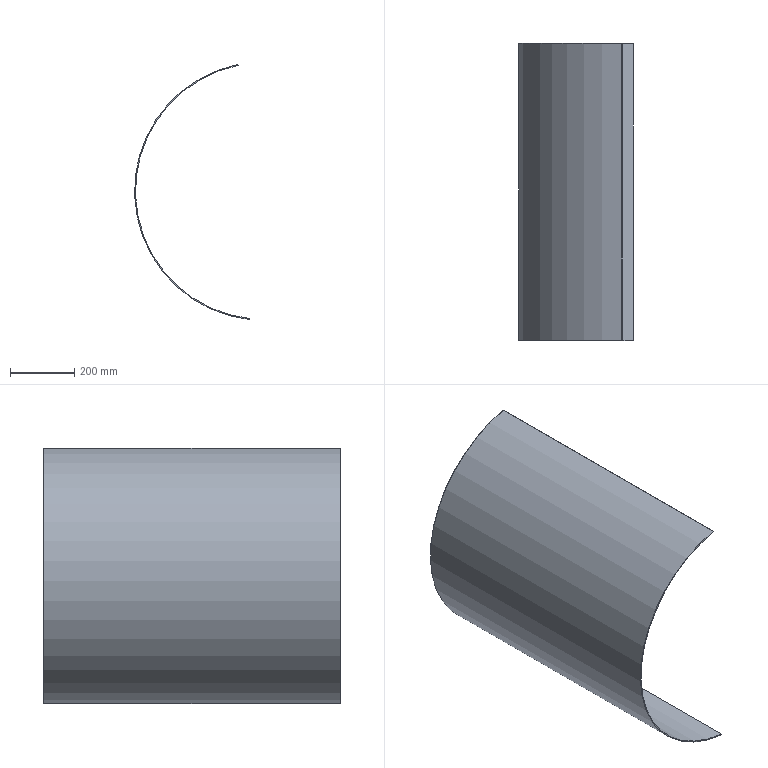Part | NX | features DATUM_CSYS 2, EXTRUDE 1, SKETCH 1 | 1 solid | 6 faces | box 358 x 926 x 795.299 mm | volume 3153696 mm3 | plane 4 | cylinder 2 | commonest cylinder face diameters 800 x1 806 x1
STEP:
#1=CARTESIAN_POINT('',(-80.,463.,391.918));
#2=VERTEX_POINT('',#1);
#3=CARTESIAN_POINT('',(-80.6,463.,394.858));
#4=VERTEX_POINT('',#3);
#5=CARTESIAN_POINT('',(-80.,463.,391.918));
#6=DIRECTION('',(-0.2,0.,0.9798));
#7=VECTOR('',#6,1000.);
#8=LINE('',#5,#7);
#9=EDGE_CURVE('',#2,#4,#8,.T.);
#10=ORIENTED_EDGE('',*,*,#9,.F.);
#11=CARTESIAN_POINT('',(-45.,463.,-397.461));
#12=VERTEX_POINT('',#11);
#13=CARTESIAN_POINT('',(0.,463.,0.));
#14=DIRECTION('',(0.,-1.,0.));
#15=DIRECTION('',(1.,0.,0.));
#16=AXIS2_PLACEMENT_3D('',#13,#14,#15);
#17=CIRCLE('',#16,400.);
#18=EDGE_CURVE('',#2,#12,#17,.T.);
#19=ORIENTED_EDGE('',*,*,#18,.T.);
#20=CARTESIAN_POINT('',(-45.338,463.,-400.442));
#21=VERTEX_POINT('',#20);
#22=CARTESIAN_POINT('',(-45.,463.,-397.461));
#23=DIRECTION('',(-0.1125,0.,-0.9937));
#24=VECTOR('',#23,1000.);
#25=LINE('',#22,#24);
#26=EDGE_CURVE('',#12,#21,#25,.T.);
#27=ORIENTED_EDGE('',*,*,#26,.T.);
#28=CARTESIAN_POINT('',(0.,463.,0.));
#29=DIRECTION('',(0.,-1.,0.));
#30=DIRECTION('',(0.,0.,-1.));
#31=AXIS2_PLACEMENT_3D('',#28,#29,#30);
#32=CIRCLE('',#31,403.);
#33=EDGE_CURVE('',#4,#21,#32,.T.);
#34=ORIENTED_EDGE('',*,*,#33,.F.);
#35=EDGE_LOOP('',(#10,#19,#27,#34));
#36=FACE_BOUND('',#35,.T.);
#37=CARTESIAN_POINT('',(0.,463.,0.));
#38=DIRECTION('',(0.,1.,0.));
#39=DIRECTION('',(0.,0.,1.));
#40=AXIS2_PLACEMENT_3D('',#37,#38,#39);
#41=PLANE('',#40);
#42=ADVANCED_FACE('',(#36),#41,.T.);
#43=ORIENTED_EDGE('',*,*,#26,.F.);
#44=CARTESIAN_POINT('',(-45.,-463.,-397.461));
#45=VERTEX_POINT('',#44);
#46=CARTESIAN_POINT('',(-45.,463.,-397.461));
#47=DIRECTION('',(0.,-1.,0.));
#48=VECTOR('',#47,1000.);
#49=LINE('',#46,#48);
#50=EDGE_CURVE('',#12,#45,#49,.T.);
#51=ORIENTED_EDGE('',*,*,#50,.T.);
#52=CARTESIAN_POINT('',(-45.338,-463.,-400.442));
#53=VERTEX_POINT('',#52);
#54=CARTESIAN_POINT('',(-45.,-463.,-397.461));
#55=DIRECTION('',(-0.1125,0.,-0.9937));
#56=VECTOR('',#55,1000.);
#57=LINE('',#54,#56);
#58=EDGE_CURVE('',#45,#53,#57,.T.);
#59=ORIENTED_EDGE('',*,*,#58,.T.);
#60=CARTESIAN_POINT('',(-45.338,463.,-400.442));
#61=DIRECTION('',(0.,-1.,0.));
#62=VECTOR('',#61,1000.);
#63=LINE('',#60,#62);
#64=EDGE_CURVE('',#21,#53,#63,.T.);
#65=ORIENTED_EDGE('',*,*,#64,.F.);
#66=EDGE_LOOP('',(#43,#51,#59,#65));
#67=FACE_BOUND('',#66,.T.);
#68=CARTESIAN_POINT('',(-45.,0.,-397.461));
#69=DIRECTION('',(0.9937,0.,-0.1125));
#70=DIRECTION('',(0.,-1.,0.));
#71=AXIS2_PLACEMENT_3D('',#68,#69,#70);
#72=PLANE('',#71);
#73=ADVANCED_FACE('',(#67),#72,.T.);
#74=ORIENTED_EDGE('',*,*,#58,.F.);
#75=CARTESIAN_POINT('',(-80.,-463.,391.918));
#76=VERTEX_POINT('',#75);
#77=CARTESIAN_POINT('',(0.,-463.,0.));
#78=DIRECTION('',(0.,-1.,0.));
#79=DIRECTION('',(1.,0.,0.));
#80=AXIS2_PLACEMENT_3D('',#77,#78,#79);
#81=CIRCLE('',#80,400.);
#82=EDGE_CURVE('',#76,#45,#81,.T.);
#83=ORIENTED_EDGE('',*,*,#82,.F.);
#84=CARTESIAN_POINT('',(-80.6,-463.,394.858));
#85=VERTEX_POINT('',#84);
#86=CARTESIAN_POINT('',(-80.,-463.,391.918));
#87=DIRECTION('',(-0.2,0.,0.9798));
#88=VECTOR('',#87,1000.);
#89=LINE('',#86,#88);
#90=EDGE_CURVE('',#76,#85,#89,.T.);
#91=ORIENTED_EDGE('',*,*,#90,.T.);
#92=CARTESIAN_POINT('',(0.,-463.,0.));
#93=DIRECTION('',(0.,-1.,0.));
#94=DIRECTION('',(0.,0.,-1.));
#95=AXIS2_PLACEMENT_3D('',#92,#93,#94);
#96=CIRCLE('',#95,403.);
#97=EDGE_CURVE('',#85,#53,#96,.T.);
#98=ORIENTED_EDGE('',*,*,#97,.T.);
#99=EDGE_LOOP('',(#74,#83,#91,#98));
#100=FACE_BOUND('',#99,.T.);
#101=CARTESIAN_POINT('',(0.,-463.,0.));
#102=DIRECTION('',(0.,1.,0.));
#103=DIRECTION('',(0.,0.,1.));
#104=AXIS2_PLACEMENT_3D('',#101,#102,#103);
#105=PLANE('',#104);
#106=ADVANCED_FACE('',(#100),#105,.F.);
#107=CARTESIAN_POINT('',(-80.,463.,391.918));
#108=DIRECTION('',(0.,-1.,0.));
#109=VECTOR('',#108,1000.);
#110=LINE('',#107,#109);
#111=EDGE_CURVE('',#2,#76,#110,.T.);
#112=ORIENTED_EDGE('',*,*,#111,.F.);
#113=ORIENTED_EDGE('',*,*,#9,.T.);
#114=CARTESIAN_POINT('',(-80.6,463.,394.858));
#115=DIRECTION('',(0.,-1.,0.));
#116=VECTOR('',#115,1000.);
#117=LINE('',#114,#116);
#118=EDGE_CURVE('',#4,#85,#117,.T.);
#119=ORIENTED_EDGE('',*,*,#118,.T.);
#120=ORIENTED_EDGE('',*,*,#90,.F.);
#121=EDGE_LOOP('',(#112,#113,#119,#120));
#122=FACE_BOUND('',#121,.T.);
#123=CARTESIAN_POINT('',(-80.,0.,391.918));
#124=DIRECTION('',(-0.9798,0.,-0.2));
#125=DIRECTION('',(0.,-1.,0.));
#126=AXIS2_PLACEMENT_3D('',#123,#124,#125);
#127=PLANE('',#126);
#128=ADVANCED_FACE('',(#122),#127,.F.);
#129=ORIENTED_EDGE('',*,*,#97,.F.);
#130=ORIENTED_EDGE('',*,*,#118,.F.);
#131=ORIENTED_EDGE('',*,*,#33,.T.);
#132=ORIENTED_EDGE('',*,*,#64,.T.);
#133=EDGE_LOOP('',(#129,#130,#131,#132));
#134=FACE_BOUND('',#133,.T.);
#135=CARTESIAN_POINT('',(0.,463.,0.));
#136=DIRECTION('',(0.,-1.,0.));
#137=DIRECTION('',(0.,0.,-1.));
#138=AXIS2_PLACEMENT_3D('',#135,#136,#137);
#139=CYLINDRICAL_SURFACE('',#138,403.);
#140=ADVANCED_FACE('',(#134),#139,.T.);
#141=ORIENTED_EDGE('',*,*,#82,.T.);
#142=ORIENTED_EDGE('',*,*,#50,.F.);
#143=ORIENTED_EDGE('',*,*,#18,.F.);
#144=ORIENTED_EDGE('',*,*,#111,.T.);
#145=EDGE_LOOP('',(#141,#142,#143,#144));
#146=FACE_BOUND('',#145,.T.);
#147=CARTESIAN_POINT('',(0.,463.,0.));
#148=DIRECTION('',(0.,-1.,0.));
#149=DIRECTION('',(0.,0.,-1.));
#150=AXIS2_PLACEMENT_3D('',#147,#148,#149);
#151=CYLINDRICAL_SURFACE('',#150,400.);
#152=ADVANCED_FACE('',(#146),#151,.F.);
#153=CLOSED_SHELL('',(#42,#73,#106,#128,#140,#152));
#154=MANIFOLD_SOLID_BREP('',#153);
#155=(LENGTH_UNIT()NAMED_UNIT(*)SI_UNIT(.MILLI.,.METRE.));
#156=UNCERTAINTY_MEASURE_WITH_UNIT(LENGTH_MEASURE(0.00001),#155,'','');
#157=(NAMED_UNIT(*)PLANE_ANGLE_UNIT()SI_UNIT($,.RADIAN.));
#158=(NAMED_UNIT(*)SI_UNIT($,.STERADIAN.)SOLID_ANGLE_UNIT());
#159=(GEOMETRIC_REPRESENTATION_CONTEXT(3)GLOBAL_UNCERTAINTY_ASSIGNED_CONTEXT((#156))GLOBAL_UNIT_ASSIGNED_CONTEXT((#155,#157,#158))REPRESENTATION_CONTEXT('',''));
#160=ADVANCED_BREP_SHAPE_REPRESENTATION('',(#154),#159);